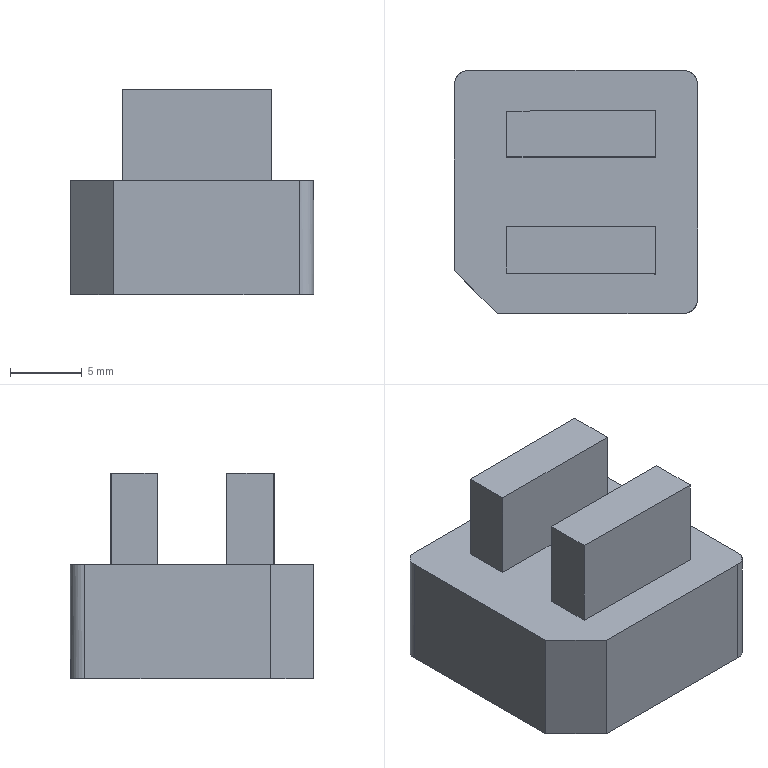NC program | PowerMill | posted with a generic post | part box 17 x 17 x 14.396 mm
Lines 1 to 1014 of 42940:
%
O0001
N104 ( POWERMILL CB  : 2026004.0)
N105 ( POST VER      : 2026.0.0.5161)
N106 ( OPTION FILE   : FANUC)
N107 ( OUTPUT WORKPLANE : WORLD)
N108 (  )
N109 ( TOOL LIST )
N110 (---------------------------------------)
N111 ( NO. | ID        | DIA.| TIP RAD|LENGTH)
N112 (---------------------------------------)
N113 (    1|D10C_1_1   |10.0 |  0.0   |69.84 )
N114 (   15|D3C_2_1    | 3.0 |  0.0   |61.44 )
N115 (    3|D10_1_1    |10.0 |  0.0   |69.56 )
N116 (   10|D3_3       | 3.0 |  0.0   |61.44 )
N117 (   13|TEXT_D4_1_1| 4.0 |  0.3   |61.64 )
N118 (---------------------------------------)
N119 (  )
N120 ( NUMBER OF TOOLPATHS: 11.0 )
N121 ( ESTIMATED PROGRAM DURATION: 0 HOURS 8 MIN 50 SEC)
N122 (  )
N123 G00 G21 G80 G40 G17
N124 G90
N125 G54
N126 G53 Z0.0
N127 (---------------)
N128 ( START TOOLPATH : 粗公开粗01-扫面平行-D10C )
N129 (---------------)
N130 ( TOOL NO.    :1 )
N131 ( TOOL TYPE   : ENDMILL)
N132 ( TOOL ID     : D10C_1_1)
N133 ( TOOL DIA    : 10.0 LENGTH 69.84)
N134 T1
N135 M6
N136 S8000 M03
N137 G00 G90 X0.0 Y0.0
N138 G43 Z10.2 H1
N139
N140 G05 P10000 R4
N141 X16.15 Y11.15
N142 Z1.198
N143 G01 Z-0.002 F6000.0
N144 X11.15 F10000.0
N145 X-11.15
N146 Y5.575
N147 X11.15
N148 Y0.0
N149 X-11.15
N150 Y-5.575
N151 X11.15
N152 Y-11.15
N153 X-11.15
N154 X-16.15
N155 Z-0.204
N156 X-11.15
N157 X11.15
N158 Y-5.575
N159 X-11.15
N160 Y0.0
N161 X11.15
N162 Y5.575
N163 X-11.15
N164 Y11.15
N165 X11.15
N166 X16.15
N167 G00 Z10.2
N168 G05 P0
N169 (---------------)
N170 ( END TOOLPATH : 粗公开粗01-扫面平行-D10C )
N171 (---------------)
N172 ( START TOOLPATH : 粗公开粗01-外形偏置-D10C )
N173 (---------------)
N174 G00 X0.3365 Y-0.0255 Z9.7958
N175 G05 P10000 R4
N176 X18.472 Y10.1346
N177 Z0.5587
N178 G01 Z-0.6413 F6000.0
N179 X17.9445 F10000.0
N180 G03 X13.197 Y5.3871 I0.0 J-4.7475
N181 G01 Y-12.389
N182 G02 X12.197 Y-13.389 I-1.0 J0.0
N183 G01 X-11.524
N184 G02 X-12.524 Y-12.389 I0.0 J1.0
N185 G01 Y12.338
N186 G02 X-11.524 Y13.338 I1.0 J0.0
N187 G01 X12.197
N188 G02 X13.197 Y12.338 I0.0 J-1.0
N189 G01 Y5.3871
N190 X10.6981 Y5.3885
N191 X10.6964 Y2.2948
N192 X10.6174 Y1.5214
N193 X10.4159 Y0.7479
N194 X10.2648 Y0.3616
N195 X10.1893 Y0.2061
N196 G03 X10.1798 Y-0.21 I0.4498 J-0.2184
N197 G01 X10.4333 Y-0.7989
N198 X10.6263 Y-1.5724
N199 X10.6974 Y-2.3458
N200 X10.6981 Y-5.4395
N201 X10.6763 Y-6.2129
N202 X10.5449 Y-6.9863
N203 X10.2853 Y-7.7598
N204 X10.0043 Y-8.321
N205 X9.8745 Y-8.5332
N206 X9.2627 Y-9.3066
N207 X8.4575 Y-9.9889
N208 X7.6841 Y-10.4256
N209 X6.9106 Y-10.7059
N210 X6.1554 Y-10.8535
N211 X5.3638 Y-10.8885
N212 X-4.6908 Y-10.8359
N213 X-5.4642 Y-10.8011
N214 X-6.2376 Y-10.6516
N215 X-7.0111 Y-10.3714
N216 X-7.5603 Y-10.08
N217 X-7.7845 Y-9.9351
N218 X-8.5375 Y-9.3066
N219 X-9.1668 Y-8.5332
N220 X-9.3313 Y-8.2684
N221 X-9.5897 Y-7.7598
N222 X-9.859 Y-6.9863
N223 X-9.9991 Y-6.2129
N224 X-10.0262 Y-5.4395
N225 X-10.0256 Y-2.3458
N226 X-9.9545 Y-1.5724
N227 X-9.7614 Y-0.7989
N228 X-9.479 Y-0.1522
N229 G03 X-9.4779 Y0.2454 I-0.4582 J0.2
N230 G01 X-9.694 Y0.7479
N231 X-9.8955 Y1.5214
N232 X-9.9744 Y2.2948
N233 X-9.9763 Y5.3885
N234 X-9.9493 Y6.1619
N235 X-9.8094 Y6.9353
N236 X-9.5404 Y7.7088
N237 X-9.3313 Y8.1307
N238 X-9.1178 Y8.4822
N239 X-8.5579 Y9.1846
N240 X-7.7845 Y9.8509
N241 X-7.5128 Y10.029
N242 X-7.0111 Y10.2989
N243 X-6.2376 Y10.5882
N244 X-5.4642 Y10.7457
N245 X-4.6908 Y10.7861
N246 X5.3638 Y10.8387
N247 X6.1372 Y10.8058
N248 X6.9106 Y10.6561
N249 X7.6841 Y10.3758
N250 X8.4575 Y9.9391
N251 X9.2309 Y9.2896
N252 X9.8753 Y8.4822
N253 X10.0043 Y8.2713
N254 X10.2859 Y7.7088
N255 X10.5452 Y6.9353
N256 X10.6764 Y6.1619
N257 X10.6981 Y5.3885
N258 X13.197 Y5.3871
N259 G00 Z3.2215
N260 G01 X18.472 Y10.1346
N261 G00 Z0.1715
N262 G01 Z-1.0285 F6000.0
N263 X17.9445 F10000.0
N264 G03 X13.197 Y5.3871 I0.0 J-4.7475
N265 G01 Y-12.389
N266 G02 X12.197 Y-13.389 I-1.0 J0.0
N267 G01 X-11.524
N268 G02 X-12.524 Y-12.389 I0.0 J1.0
N269 G01 Y12.338
N270 G02 X-11.524 Y13.338 I1.0 J0.0
N271 G01 X12.197
N272 G02 X13.197 Y12.338 I0.0 J-1.0
N273 G01 Y5.3871
N274 X10.6981 Y5.3885
N275 X10.6964 Y2.2948
N276 X10.6174 Y1.5214
N277 X10.4159 Y0.7479
N278 X10.2648 Y0.3616
N279 X10.1893 Y0.2061
N280 G03 X10.1798 Y-0.21 I0.4498 J-0.2184
N281 G01 X10.4334 Y-0.7989
N282 X10.6263 Y-1.5724
N283 X10.6974 Y-2.3458
N284 X10.6981 Y-5.4395
N285 X10.6763 Y-6.2129
N286 X10.5449 Y-6.9863
N287 X10.2853 Y-7.7598
N288 X10.0043 Y-8.321
N289 X9.8745 Y-8.5332
N290 X9.2627 Y-9.3066
N291 X8.4575 Y-9.9889
N292 X7.6841 Y-10.4256
N293 X6.9106 Y-10.7059
N294 X6.1554 Y-10.8535
N295 X5.3638 Y-10.8885
N296 X-4.6908 Y-10.8359
N297 X-5.4642 Y-10.8011
N298 X-6.2376 Y-10.6516
N299 X-7.0111 Y-10.3714
N300 X-7.5603 Y-10.08
N301 X-7.7845 Y-9.9351
N302 X-8.5375 Y-9.3066
N303 X-9.1668 Y-8.5332
N304 X-9.3313 Y-8.2684
N305 X-9.5897 Y-7.7598
N306 X-9.859 Y-6.9863
N307 X-9.9991 Y-6.2129
N308 X-10.0263 Y-5.4395
N309 X-10.0256 Y-2.3458
N310 X-9.9545 Y-1.5724
N311 X-9.7614 Y-0.7989
N312 X-9.479 Y-0.1522
N313 G03 X-9.4779 Y0.2454 I-0.4582 J0.2
N314 G01 X-9.694 Y0.7479
N315 X-9.8956 Y1.5214
N316 X-9.9744 Y2.2948
N317 X-9.9763 Y5.3885
N318 X-9.9493 Y6.1619
N319 X-9.8094 Y6.9353
N320 X-9.5404 Y7.7088
N321 X-9.3313 Y8.1307
N322 X-9.1178 Y8.4822
N323 X-8.5579 Y9.1846
N324 X-7.7845 Y9.8509
N325 X-7.5128 Y10.029
N326 X-7.0111 Y10.2989
N327 X-6.2376 Y10.5882
N328 X-5.4642 Y10.7457
N329 X-4.6908 Y10.7861
N330 X5.3638 Y10.8387
N331 X6.1372 Y10.8058
N332 X6.9106 Y10.6561
N333 X7.6841 Y10.3758
N334 X8.4575 Y9.9392
N335 X9.2309 Y9.2896
N336 X9.8753 Y8.4822
N337 X10.0043 Y8.2713
N338 X10.2859 Y7.7088
N339 X10.5452 Y6.9353
N340 X10.6764 Y6.1619
N341 X10.6981 Y5.3885
N342 X13.197 Y5.3871
N343 G00 Z2.8342
N344 G01 X18.472 Y10.1346
N345 G00 Z-0.2158
N346 G01 Z-1.4158 F6000.0
N347 X17.9445 F10000.0
N348 G03 X13.197 Y5.3871 I0.0 J-4.7475
N349 G01 Y-12.389
N350 G02 X12.197 Y-13.389 I-1.0 J0.0
N351 G01 X-11.524
N352 G02 X-12.524 Y-12.389 I0.0 J1.0
N353 G01 Y12.338
N354 G02 X-11.524 Y13.338 I1.0 J0.0
N355 G01 X12.197
N356 G02 X13.197 Y12.338 I0.0 J-1.0
N357 G01 Y5.3871
N358 X10.6981 Y5.3885
N359 X10.6964 Y2.2948
N360 X10.6174 Y1.5214
N361 X10.4159 Y0.7479
N362 X10.2648 Y0.3616
N363 X10.1893 Y0.2061
N364 G03 X10.1798 Y-0.2101 I0.4498 J-0.2184
N365 G01 X10.4334 Y-0.7989
N366 X10.6263 Y-1.5724
N367 X10.6974 Y-2.3458
N368 X10.6981 Y-5.4395
N369 X10.6763 Y-6.2129
N370 X10.5449 Y-6.9863
N371 X10.2853 Y-7.7598
N372 X10.0043 Y-8.321
N373 X9.8745 Y-8.5332
N374 X9.2627 Y-9.3066
N375 X8.4575 Y-9.9889
N376 X7.6841 Y-10.4256
N377 X6.9106 Y-10.7059
N378 X6.1554 Y-10.8535
N379 X5.3638 Y-10.8885
N380 X-4.6908 Y-10.8359
N381 X-5.4642 Y-10.8011
N382 X-6.2376 Y-10.6516
N383 X-7.0111 Y-10.3715
N384 X-7.5603 Y-10.08
N385 X-7.7845 Y-9.9351
N386 X-8.5375 Y-9.3066
N387 X-9.1668 Y-8.5332
N388 X-9.3313 Y-8.2684
N389 X-9.5897 Y-7.7598
N390 X-9.8591 Y-6.9863
N391 X-9.9991 Y-6.2129
N392 X-10.0263 Y-5.4395
N393 X-10.0256 Y-2.3458
N394 X-9.9545 Y-1.5724
N395 X-9.7614 Y-0.7989
N396 X-9.479 Y-0.1522
N397 G03 X-9.4779 Y0.2454 I-0.4582 J0.2
N398 G01 X-9.694 Y0.7479
N399 X-9.8956 Y1.5214
N400 X-9.9744 Y2.2948
N401 X-9.9763 Y5.3885
N402 X-9.9493 Y6.1619
N403 X-9.8094 Y6.9353
N404 X-9.5404 Y7.7088
N405 X-9.3313 Y8.1307
N406 X-9.1178 Y8.4822
N407 X-8.5579 Y9.1846
N408 X-7.7845 Y9.8509
N409 X-7.5128 Y10.029
N410 X-7.0111 Y10.299
N411 X-6.2376 Y10.5882
N412 X-5.4642 Y10.7457
N413 X-4.6908 Y10.7861
N414 X5.3638 Y10.8387
N415 X6.1372 Y10.8058
N416 X6.9106 Y10.6561
N417 X7.6841 Y10.3758
N418 X8.4575 Y9.9392
N419 X9.2309 Y9.2896
N420 X9.8753 Y8.4822
N421 X10.0043 Y8.2713
N422 X10.2859 Y7.7088
N423 X10.5452 Y6.9353
N424 X10.6764 Y6.1619
N425 X10.6981 Y5.3885
N426 X13.197 Y5.3871
N427 G00 Z2.447
N428 G01 X18.472 Y10.1346
N429 G00 Z-0.603
N430 G01 Z-1.803 F6000.0
N431 X17.9445 F10000.0
N432 G03 X13.197 Y5.3871 I0.0 J-4.7475
N433 G01 Y-12.389
N434 G02 X12.197 Y-13.389 I-1.0 J0.0
N435 G01 X-11.524
N436 G02 X-12.524 Y-12.389 I0.0 J1.0
N437 G01 Y12.338
N438 G02 X-11.524 Y13.338 I1.0 J0.0
N439 G01 X12.197
N440 G02 X13.197 Y12.338 I0.0 J-1.0
N441 G01 Y5.3871
N442 X10.6981 Y5.3885
N443 X10.6964 Y2.2948
N444 X10.6174 Y1.5214
N445 X10.4159 Y0.7479
N446 X10.2648 Y0.3616
N447 X10.1893 Y0.2061
N448 G03 X10.1798 Y-0.2101 I0.4498 J-0.2184
N449 G01 X10.4334 Y-0.7989
N450 X10.6263 Y-1.5724
N451 X10.6974 Y-2.3458
N452 X10.6981 Y-5.4395
N453 X10.6763 Y-6.2129
N454 X10.545 Y-6.9863
N455 X10.2853 Y-7.7598
N456 X10.0043 Y-8.321
N457 X9.8745 Y-8.5332
N458 X9.2627 Y-9.3066
N459 X8.4575 Y-9.9889
N460 X7.6841 Y-10.4256
N461 X6.9106 Y-10.7059
N462 X6.1554 Y-10.8535
N463 X5.3638 Y-10.8885
N464 X-4.6908 Y-10.8359
N465 X-5.4642 Y-10.8011
N466 X-6.2376 Y-10.6516
N467 X-7.0111 Y-10.3715
N468 X-7.5603 Y-10.08
N469 X-7.7845 Y-9.9351
N470 X-8.5375 Y-9.3066
N471 X-9.1668 Y-8.5332
N472 X-9.3313 Y-8.2684
N473 X-9.5897 Y-7.7598
N474 X-9.8591 Y-6.9863
N475 X-9.9991 Y-6.2129
N476 X-10.0263 Y-5.4395
N477 X-10.0256 Y-2.3458
N478 X-9.9545 Y-1.5724
N479 X-9.7614 Y-0.7989
N480 X-9.479 Y-0.1522
N481 G03 X-9.4779 Y0.2454 I-0.4582 J0.2
N482 G01 X-9.694 Y0.7479
N483 X-9.8956 Y1.5214
N484 X-9.9745 Y2.2948
N485 X-9.9763 Y5.3885
N486 X-9.9493 Y6.1619
N487 X-9.8094 Y6.9353
N488 X-9.5404 Y7.7088
N489 X-9.3313 Y8.1307
N490 X-9.1178 Y8.4822
N491 X-8.5579 Y9.1846
N492 X-7.7845 Y9.8509
N493 X-7.5128 Y10.029
N494 X-7.0111 Y10.299
N495 X-6.2376 Y10.5882
N496 X-5.4642 Y10.7457
N497 X-4.6908 Y10.7861
N498 X5.3638 Y10.8387
N499 X6.1372 Y10.8058
N500 X6.9106 Y10.6561
N501 X7.6841 Y10.3758
N502 X8.4575 Y9.9392
N503 X9.2309 Y9.2896
N504 X9.8753 Y8.4822
N505 X10.0043 Y8.2713
N506 X10.2859 Y7.7088
N507 X10.5452 Y6.9353
N508 X10.6764 Y6.1619
N509 X10.6981 Y5.3885
N510 X13.197 Y5.3871
N511 G00 Z2.0598
N512 G01 X18.472 Y10.1346
N513 G00 Z-0.9902
N514 G01 Z-2.1902 F6000.0
N515 X17.9445 F10000.0
N516 G03 X13.197 Y5.3871 I0.0 J-4.7475
N517 G01 Y-12.389
N518 G02 X12.197 Y-13.389 I-1.0 J0.0
N519 G01 X-11.524
N520 G02 X-12.524 Y-12.389 I0.0 J1.0
N521 G01 Y12.338
N522 G02 X-11.524 Y13.338 I1.0 J0.0
N523 G01 X12.197
N524 G02 X13.197 Y12.338 I0.0 J-1.0
N525 G01 Y5.3871
N526 X10.6981 Y5.3885
N527 X10.6964 Y2.2948
N528 X10.6174 Y1.5214
N529 X10.4159 Y0.7479
N530 X10.2648 Y0.3616
N531 X10.1893 Y0.2061
N532 G03 X10.1798 Y-0.2101 I0.4498 J-0.2184
N533 G01 X10.4334 Y-0.7989
N534 X10.6264 Y-1.5724
N535 X10.6975 Y-2.3458
N536 X10.6981 Y-5.4395
N537 X10.6763 Y-6.2129
N538 X10.545 Y-6.9863
N539 X10.2853 Y-7.7598
N540 X10.0043 Y-8.321
N541 X9.8745 Y-8.5332
N542 X9.2627 Y-9.3066
N543 X8.4575 Y-9.9889
N544 X7.6841 Y-10.4256
N545 X6.9106 Y-10.7059
N546 X6.1554 Y-10.8535
N547 X5.3638 Y-10.8885
N548 X-4.6908 Y-10.8359
N549 X-5.4642 Y-10.8011
N550 X-6.2376 Y-10.6516
N551 X-7.0111 Y-10.3715
N552 X-7.5603 Y-10.08
N553 X-7.7845 Y-9.9351
N554 X-8.5375 Y-9.3066
N555 X-9.1668 Y-8.5332
N556 X-9.3313 Y-8.2684
N557 X-9.5897 Y-7.7598
N558 X-9.8591 Y-6.9863
N559 X-9.9991 Y-6.2129
N560 X-10.0263 Y-5.4395
N561 X-10.0256 Y-2.3458
N562 X-9.9545 Y-1.5724
N563 X-9.7614 Y-0.7989
N564 X-9.479 Y-0.1522
N565 G03 X-9.4779 Y0.2454 I-0.4582 J0.2
N566 G01 X-9.694 Y0.7479
N567 X-9.8956 Y1.5214
N568 X-9.9745 Y2.2948
N569 X-9.9763 Y5.3885
N570 X-9.9493 Y6.1619
N571 X-9.8094 Y6.9353
N572 X-9.5404 Y7.7088
N573 X-9.3313 Y8.1307
N574 X-9.1179 Y8.4822
N575 X-8.5579 Y9.1846
N576 X-7.7845 Y9.8509
N577 X-7.5129 Y10.029
N578 X-7.0111 Y10.299
N579 X-6.2376 Y10.5882
N580 X-5.4642 Y10.7457
N581 X-4.6908 Y10.7861
N582 X5.3638 Y10.8387
N583 X6.1372 Y10.8058
N584 X6.9106 Y10.6561
N585 X7.6841 Y10.3758
N586 X8.4575 Y9.9392
N587 X9.2309 Y9.2896
N588 X9.8753 Y8.4822
N589 X10.0043 Y8.2713
N590 X10.2859 Y7.7088
N591 X10.5452 Y6.9353
N592 X10.6764 Y6.1619
N593 X10.6981 Y5.3885
N594 X13.197 Y5.3871
N595 G00 Z1.6725
N596 G01 X18.472 Y10.1346
N597 G00 Z-1.3775
N598 G01 Z-2.5775 F6000.0
N599 X17.9445 F10000.0
N600 G03 X13.197 Y5.3871 I0.0 J-4.7475
N601 G01 Y-12.389
N602 G02 X12.197 Y-13.389 I-1.0 J0.0
N603 G01 X-11.524
N604 G02 X-12.524 Y-12.389 I0.0 J1.0
N605 G01 Y12.338
N606 G02 X-11.524 Y13.338 I1.0 J0.0
N607 G01 X12.197
N608 G02 X13.197 Y12.338 I0.0 J-1.0
N609 G01 Y5.3871
N610 X10.6982 Y5.3885
N611 X10.6964 Y2.2948
N612 X10.6174 Y1.5214
N613 X10.4159 Y0.7479
N614 X10.2648 Y0.3616
N615 X10.1893 Y0.2061
N616 G03 X10.1798 Y-0.2101 I0.4498 J-0.2184
N617 G01 X10.4334 Y-0.7989
N618 X10.6264 Y-1.5724
N619 X10.6975 Y-2.3458
N620 X10.6982 Y-5.4395
N621 X10.6764 Y-6.2129
N622 X10.545 Y-6.9863
N623 X10.2853 Y-7.7598
N624 X10.0043 Y-8.321
N625 X9.8745 Y-8.5332
N626 X9.2627 Y-9.3066
N627 X8.4575 Y-9.989
N628 X7.6841 Y-10.4256
N629 X6.9106 Y-10.7059
N630 X6.1554 Y-10.8535
N631 X5.3638 Y-10.8885
N632 X-4.6908 Y-10.8359
N633 X-5.4642 Y-10.8012
N634 X-6.2376 Y-10.6516
N635 X-7.0111 Y-10.3715
N636 X-7.5603 Y-10.08
N637 X-7.7845 Y-9.9351
N638 X-8.5375 Y-9.3066
N639 X-9.1668 Y-8.5332
N640 X-9.3313 Y-8.2684
N641 X-9.5897 Y-7.7598
N642 X-9.8591 Y-6.9863
N643 X-9.9991 Y-6.2129
N644 X-10.0263 Y-5.4395
N645 X-10.0256 Y-2.3458
N646 X-9.9545 Y-1.5724
N647 X-9.7614 Y-0.7989
N648 X-9.479 Y-0.1523
N649 G03 X-9.4779 Y0.2454 I-0.4582 J0.2001
N650 G01 X-9.694 Y0.7479
N651 X-9.8956 Y1.5214
N652 X-9.9745 Y2.2948
N653 X-9.9763 Y5.3885
N654 X-9.9493 Y6.1619
N655 X-9.8094 Y6.9353
N656 X-9.5404 Y7.7088
N657 X-9.3313 Y8.1307
N658 X-9.1179 Y8.4822
N659 X-8.5579 Y9.1846
N660 X-7.7845 Y9.8509
N661 X-7.5129 Y10.029
N662 X-7.0111 Y10.299
N663 X-6.2376 Y10.5882
N664 X-5.4642 Y10.7457
N665 X-4.6908 Y10.7861
N666 X5.3638 Y10.8388
N667 X6.1372 Y10.8059
N668 X6.9106 Y10.6562
N669 X7.6841 Y10.3758
N670 X8.4575 Y9.9392
N671 X9.2309 Y9.2896
N672 X9.8753 Y8.4822
N673 X10.0043 Y8.2713
N674 X10.2859 Y7.7088
N675 X10.5452 Y6.9353
N676 X10.6764 Y6.1619
N677 X10.6982 Y5.3885
N678 X13.197 Y5.3871
N679 G00 Z1.2852
N680 G01 X18.472 Y10.1346
N681 G00 Z-1.7648
N682 G01 Z-2.9648 F6000.0
N683 X17.9445 F10000.0
N684 G03 X13.197 Y5.3871 I0.0 J-4.7475
N685 G01 Y-12.389
N686 G02 X12.197 Y-13.389 I-1.0 J0.0
N687 G01 X-11.524
N688 G02 X-12.524 Y-12.389 I0.0 J1.0
N689 G01 Y12.338
N690 G02 X-11.524 Y13.338 I1.0 J0.0
N691 G01 X12.197
N692 G02 X13.197 Y12.338 I0.0 J-1.0
N693 G01 Y5.3871
N694 X10.6982 Y5.3885
N695 X10.6964 Y2.2948
N696 X10.6175 Y1.5214
N697 X10.4159 Y0.7479
N698 X10.2648 Y0.3616
N699 X10.1893 Y0.2061
N700 G03 X10.1798 Y-0.2101 I0.4498 J-0.2184
N701 G01 X10.4334 Y-0.7989
N702 X10.6264 Y-1.5724
N703 X10.6975 Y-2.3458
N704 X10.6982 Y-5.4395
N705 X10.6764 Y-6.2129
N706 X10.545 Y-6.9863
N707 X10.2853 Y-7.7598
N708 X10.0043 Y-8.321
N709 X9.8745 Y-8.5332
N710 X9.2627 Y-9.3066
N711 X8.4575 Y-9.989
N712 X7.6841 Y-10.4256
N713 X6.9106 Y-10.7059
N714 X6.1555 Y-10.8535
N715 X5.3638 Y-10.8885
N716 X-4.6908 Y-10.8359
N717 X-5.4642 Y-10.8012
N718 X-6.2376 Y-10.6516
N719 X-7.0111 Y-10.3715
N720 X-7.5603 Y-10.08
N721 X-7.7845 Y-9.9351
N722 X-8.5375 Y-9.3066
N723 X-9.1668 Y-8.5332
N724 X-9.3313 Y-8.2684
N725 X-9.5897 Y-7.7598
N726 X-9.8591 Y-6.9863
N727 X-9.9991 Y-6.2129
N728 X-10.0263 Y-5.4395
N729 X-10.0256 Y-2.3458
N730 X-9.9545 Y-1.5724
N731 X-9.7614 Y-0.7989
N732 X-9.479 Y-0.1523
N733 G03 X-9.4779 Y0.2454 I-0.4582 J0.2001
N734 G01 X-9.694 Y0.7479
N735 X-9.8956 Y1.5214
N736 X-9.9745 Y2.2948
N737 X-9.9763 Y5.3885
N738 X-9.9493 Y6.1619
N739 X-9.8094 Y6.9353
N740 X-9.5404 Y7.7088
N741 X-9.3313 Y8.1307
N742 X-9.1179 Y8.4822
N743 X-8.5579 Y9.1846
N744 X-7.7845 Y9.8509
N745 X-7.5129 Y10.029
N746 X-7.0111 Y10.299
N747 X-6.2376 Y10.5882
N748 X-5.4642 Y10.7457
N749 X-4.6908 Y10.7861
N750 X5.3638 Y10.8388
N751 X6.1372 Y10.8059
N752 X6.9106 Y10.6562
N753 X7.6841 Y10.3758
N754 X8.4575 Y9.9392
N755 X9.2309 Y9.2896
N756 X9.8753 Y8.4822
N757 X10.0043 Y8.2714
N758 X10.2859 Y7.7088
N759 X10.5452 Y6.9353
N760 X10.6764 Y6.1619
N761 X10.6982 Y5.3885
N762 X13.197 Y5.3871
N763 G00 Z0.898
N764 G01 X18.472 Y10.1346
N765 G00 Z-2.152
N766 G01 Z-3.352 F6000.0
N767 X17.9445 F10000.0
N768 G03 X13.197 Y5.3871 I0.0 J-4.7475
N769 G01 Y-12.389
N770 G02 X12.197 Y-13.389 I-1.0 J0.0
N771 G01 X-11.524
N772 G02 X-12.524 Y-12.389 I0.0 J1.0
N773 G01 Y12.338
N774 G02 X-11.524 Y13.338 I1.0 J0.0
N775 G01 X12.197
N776 G02 X13.197 Y12.338 I0.0 J-1.0
N777 G01 Y5.3871
N778 X10.6982 Y5.3885
N779 X10.6964 Y2.2948
N780 X10.6175 Y1.5214
N781 X10.4159 Y0.7479
N782 X10.2648 Y0.3616
N783 X10.1893 Y0.2061
N784 G03 X10.1798 Y-0.2101 I0.4498 J-0.2184
N785 G01 X10.4334 Y-0.7989
N786 X10.6264 Y-1.5724
N787 X10.6975 Y-2.3458
N788 X10.6982 Y-5.4395
N789 X10.6764 Y-6.2129
N790 X10.545 Y-6.9863
N791 X10.2853 Y-7.7598
N792 X10.0043 Y-8.3211
N793 X9.8745 Y-8.5332
N794 X9.2627 Y-9.3066
N795 X8.4575 Y-9.989
N796 X7.6841 Y-10.4256
N797 X6.9106 Y-10.7059
N798 X6.1555 Y-10.8535
N799 X5.3638 Y-10.8885
N800 X-4.6908 Y-10.8359
N801 X-5.4642 Y-10.8012
N802 X-6.2376 Y-10.6516
N803 X-7.0111 Y-10.3715
N804 X-7.5604 Y-10.08
N805 X-7.7845 Y-9.9351
N806 X-8.5375 Y-9.3066
N807 X-9.1668 Y-8.5332
N808 X-9.3313 Y-8.2684
N809 X-9.5897 Y-7.7598
N810 X-9.8591 Y-6.9863
N811 X-9.9991 Y-6.2129
N812 X-10.0263 Y-5.4395
N813 X-10.0256 Y-2.3458
N814 X-9.9545 Y-1.5724
N815 X-9.7614 Y-0.7989
N816 X-9.479 Y-0.1523
N817 G03 X-9.4779 Y0.2454 I-0.4583 J0.2001
N818 G01 X-9.694 Y0.7479
N819 X-9.8956 Y1.5214
N820 X-9.9745 Y2.2948
N821 X-9.9763 Y5.3885
N822 X-9.9493 Y6.1619
N823 X-9.8094 Y6.9353
N824 X-9.5404 Y7.7088
N825 X-9.3313 Y8.1307
N826 X-9.1179 Y8.4822
N827 X-8.5579 Y9.1846
N828 X-7.7845 Y9.8509
N829 X-7.5129 Y10.029
N830 X-7.0111 Y10.299
N831 X-6.2376 Y10.5882
N832 X-5.4642 Y10.7457
N833 X-4.6908 Y10.7861
N834 X5.3638 Y10.8388
N835 X6.1372 Y10.8059
N836 X6.9106 Y10.6562
N837 X7.6841 Y10.3758
N838 X8.4575 Y9.9392
N839 X9.2309 Y9.2897
N840 X9.8753 Y8.4822
N841 X10.0043 Y8.2714
N842 X10.2859 Y7.7088
N843 X10.5452 Y6.9353
N844 X10.6765 Y6.1619
N845 X10.6982 Y5.3885
N846 X13.197 Y5.3871
N847 G00 Z0.5108
N848 G01 X18.472 Y10.1346
N849 G00 Z-2.5392
N850 G01 Z-3.7392 F6000.0
N851 X17.9445 F10000.0
N852 G03 X13.197 Y5.3871 I0.0 J-4.7475
N853 G01 Y-12.389
N854 G02 X12.197 Y-13.389 I-1.0 J0.0
N855 G01 X-11.524
N856 G02 X-12.524 Y-12.389 I0.0 J1.0
N857 G01 Y12.338
N858 G02 X-11.524 Y13.338 I1.0 J0.0
N859 G01 X12.197
N860 G02 X13.197 Y12.338 I0.0 J-1.0
N861 G01 Y5.3871
N862 X10.6982 Y5.3885
N863 X10.6964 Y2.2948
N864 X10.6175 Y1.5214
N865 X10.4159 Y0.7479
N866 X10.2648 Y0.3616
N867 X10.1893 Y0.2061
N868 G03 X10.1798 Y-0.2101 I0.4498 J-0.2184
N869 G01 X10.4334 Y-0.7989
N870 X10.6264 Y-1.5724
N871 X10.6975 Y-2.3458
N872 X10.6982 Y-5.4395
N873 X10.6764 Y-6.2129
N874 X10.545 Y-6.9863
N875 X10.2853 Y-7.7598
N876 X10.0043 Y-8.3211
N877 X9.8745 Y-8.5332
N878 X9.2627 Y-9.3066
N879 X8.4575 Y-9.989
N880 X7.6841 Y-10.4256
N881 X6.9106 Y-10.706
N882 X6.1555 Y-10.8535
N883 X5.3638 Y-10.8885
N884 X-4.6908 Y-10.8359
N885 X-5.4642 Y-10.8012
N886 X-6.2376 Y-10.6516
N887 X-7.0111 Y-10.3715
N888 X-7.5604 Y-10.08
N889 X-7.7845 Y-9.9351
N890 X-8.5375 Y-9.3066
N891 X-9.1668 Y-8.5332
N892 X-9.3313 Y-8.2684
N893 X-9.5897 Y-7.7598
N894 X-9.8591 Y-6.9863
N895 X-9.9991 Y-6.2129
N896 X-10.0263 Y-5.4395
N897 X-10.0256 Y-2.3458
N898 X-9.9545 Y-1.5724
N899 X-9.7614 Y-0.7989
N900 X-9.479 Y-0.1523
N901 G03 X-9.4779 Y0.2454 I-0.4583 J0.2001
N902 G01 X-9.694 Y0.7479
N903 X-9.8956 Y1.5214
N904 X-9.9745 Y2.2948
N905 X-9.9763 Y5.3885
N906 X-9.9493 Y6.1619
N907 X-9.8094 Y6.9353
N908 X-9.5404 Y7.7088
N909 X-9.3313 Y8.1307
N910 X-9.1179 Y8.4822
N911 X-8.5579 Y9.1846
N912 X-7.7845 Y9.8509
N913 X-7.5129 Y10.029
N914 X-7.0111 Y10.299
N915 X-6.2376 Y10.5882
N916 X-5.4642 Y10.7457
N917 X-4.6908 Y10.7861
N918 X5.3638 Y10.8388
N919 X6.1372 Y10.8059
N920 X6.9106 Y10.6562
N921 X7.6841 Y10.3758
N922 X8.4575 Y9.9392
N923 X9.2309 Y9.2897
N924 X9.8753 Y8.4822
N925 X10.0043 Y8.2714
N926 X10.2859 Y7.7088
N927 X10.5452 Y6.9353
N928 X10.6765 Y6.1619
N929 X10.6982 Y5.3885
N930 X13.197 Y5.3871
N931 G00 Z0.1235
N932 G01 X18.472 Y10.1346
N933 G00 Z-2.9265
N934 G01 Z-4.1265 F6000.0
N935 X17.9445 F10000.0
N936 G03 X13.197 Y5.3871 I0.0 J-4.7475
N937 G01 Y-12.389
N938 G02 X12.197 Y-13.389 I-1.0 J0.0
N939 G01 X-11.524
N940 G02 X-12.524 Y-12.389 I0.0 J1.0
N941 G01 Y12.338
N942 G02 X-11.524 Y13.338 I1.0 J0.0
N943 G01 X12.197
N944 G02 X13.197 Y12.338 I0.0 J-1.0
N945 G01 Y5.3871
N946 X10.6982 Y5.3885
N947 X10.6964 Y2.2948
N948 X10.6175 Y1.5214
N949 X10.4159 Y0.7479
N950 X10.2648 Y0.3616
N951 X10.1893 Y0.2061
N952 G03 X10.1798 Y-0.2101 I0.4498 J-0.2184
N953 G01 X10.4334 Y-0.7989
N954 X10.6264 Y-1.5724
N955 X10.6975 Y-2.3458
N956 X10.6982 Y-5.4395
N957 X10.6764 Y-6.2129
N958 X10.545 Y-6.9863
N959 X10.2853 Y-7.7598
N960 X10.0043 Y-8.3211
N961 X9.8745 Y-8.5332
N962 X9.2627 Y-9.3066
N963 X8.4575 Y-9.989
N964 X7.6841 Y-10.4256
N965 X6.9106 Y-10.706
N966 X6.1555 Y-10.8535
N967 X5.3638 Y-10.8886
N968 X-4.6908 Y-10.8359
N969 X-5.4642 Y-10.8012
N970 X-6.2376 Y-10.6516
N971 X-7.0111 Y-10.3715
N972 X-7.5604 Y-10.08
N973 X-7.7845 Y-9.9351
N974 X-8.5376 Y-9.3066
N975 X-9.1668 Y-8.5332
N976 X-9.3313 Y-8.2684
N977 X-9.5897 Y-7.7598
N978 X-9.8591 Y-6.9863
N979 X-9.9991 Y-6.2129
N980 X-10.0263 Y-5.4395
N981 X-10.0256 Y-2.3458
N982 X-9.9545 Y-1.5724
N983 X-9.7614 Y-0.7989
N984 X-9.479 Y-0.1523
N985 G03 X-9.4779 Y0.2454 I-0.4583 J0.2001
N986 G01 X-9.6941 Y0.7479
N987 X-9.8956 Y1.5214
N988 X-9.9745 Y2.2948
N989 X-9.9763 Y5.3885
N990 X-9.9493 Y6.1619
N991 X-9.8094 Y6.9353
N992 X-9.5404 Y7.7088
N993 X-9.3313 Y8.1307
N994 X-9.1179 Y8.4822
N995 X-8.5579 Y9.1846
N996 X-7.7845 Y9.8509
N997 X-7.5129 Y10.029
N998 X-7.0111 Y10.299
N999 X-6.2376 Y10.5882
N1000 X-5.4642 Y10.7457
N1001 X-4.6908 Y10.7861
N1002 X5.3638 Y10.8388
N1003 X6.1372 Y10.8059
N1004 X6.9106 Y10.6562
N1005 X7.6841 Y10.3758
N1006 X8.4575 Y9.9392
N1007 X9.2309 Y9.2897
N1008 X9.8753 Y8.4822
N1009 X10.0043 Y8.2714
N1010 X10.2859 Y7.7088
N1011 X10.5452 Y6.9353
N1012 X10.6765 Y6.1619
N1013 X10.6982 Y5.3885
N1014 X13.197 Y5.3871
N1015 G00 Z-0.2638
N1016 G01 X18.472 Y10.1346
N1017 G00 Z-3.3138
N1018 G01 Z-4.5138 F6000.0
N1019 X17.9445 F10000.0
N1020 G03 X13.197 Y5.3871 I0.0 J-4.7475
N1021 G01 Y-12.389
N1022 G02 X12.197 Y-13.389 I-1.0 J0.0
N1023 G01 X-11.524
N1024 G02 X-12.524 Y-12.389 I0.0 J1.0
N1025 G01 Y12.338
N1026 G02 X-11.524 Y13.338 I1.0 J0.0
N1027 G01 X12.197
N1028 G02 X13.197 Y12.338 I0.0 J-1.0
N1029 G01 Y5.3871
N1030 X10.6982 Y5.3885
N1031 X10.6964 Y2.2948
N1032 X10.6175 Y1.5214
N1033 X10.4159 Y0.7479
N1034 X10.2648 Y0.3616
N1035 X10.1893 Y0.2061
N1036 G03 X10.1798 Y-0.2101 I0.4498 J-0.2184
N1037 G01 X10.4334 Y-0.7989
N1038 X10.6264 Y-1.5724
N1039 X10.6975 Y-2.3458
N1040 X10.6982 Y-5.4395
N1041 X10.6764 Y-6.2129
N1042 X10.545 Y-6.9863
N1043 X10.2853 Y-7.7598
N1044 X10.0043 Y-8.3211
N1045 X9.8745 Y-8.5332
N1046 X9.2627 Y-9.3066
N1047 X8.4575 Y-9.989
N1048 X7.6841 Y-10.4256
N1049 X6.9106 Y-10.706
N1050 X6.1555 Y-10.8535
N1051 X5.3638 Y-10.8886
N1052 X-4.6908 Y-10.8359
N1053 X-5.4642 Y-10.8012
N1054 X-6.2376 Y-10.6517
N1055 X-7.0111 Y-10.3715
N1056 X-7.5604 Y-10.08
N1057 X-7.7845 Y-9.9351
N1058 X-8.5376 Y-9.3066
N1059 X-9.1668 Y-8.5332
N1060 X-9.3313 Y-8.2684
N1061 X-9.5897 Y-7.7598
N1062 X-9.8591 Y-6.9863
N1063 X-9.9991 Y-6.2129
N1064 X-10.0263 Y-5.4395
N1065 X-10.0256 Y-2.3458
N1066 X-9.9545 Y-1.5724
N1067 X-9.7614 Y-0.7989
N1068 X-9.479 Y-0.1523
N1069 G03 X-9.4779 Y0.2454 I-0.4583 J0.2001
N1070 G01 X-9.6941 Y0.7479
N1071 X-9.8956 Y1.5214
N1072 X-9.9745 Y2.2948
N1073 X-9.9763 Y5.3885
N1074 X-9.9493 Y6.1619
N1075 X-9.8094 Y6.9353
N1076 X-9.5404 Y7.7088
N1077 X-9.3313 Y8.1307
N1078 X-9.1179 Y8.4822
N1079 X-8.5579 Y9.1846
N1080 X-7.7845 Y9.8509
N1081 X-7.5129 Y10.029
N1082 X-7.0111 Y10.299
N1083 X-6.2376 Y10.5882
N1084 X-5.4642 Y10.7457
N1085 X-4.6908 Y10.7861
N1086 X5.3638 Y10.8388
N1087 X6.1372 Y10.8059
N1088 X6.9106 Y10.6562
N1089 X7.6841 Y10.3758
N1090 X8.4575 Y9.9392
N1091 X9.2309 Y9.2897
N1092 X9.8753 Y8.4822
N1093 X10.0043 Y8.2714
N1094 X10.2859 Y7.7088
N1095 X10.5452 Y6.9353
N1096 X10.6765 Y6.1619
N1097 X10.6982 Y5.3885
N1098 X13.197 Y5.3871
N1099 G00 Z-0.651
N1100 G01 X18.472 Y10.1346
N1101 G00 Z-3.701
N1102 G01 Z-4.901 F6000.0
N1103 X17.9445 F10000.0
N1104 G03 X13.197 Y5.3871 I0.0 J-4.7475
N1105 G01 Y-12.389
N1106 G02 X12.197 Y-13.389 I-1.0 J0.0
N1107 G01 X-11.524
N1108 G02 X-12.524 Y-12.389 I0.0 J1.0
N1109 G01 Y12.338
N1110 G02 X-11.524 Y13.338 I1.0 J0.0
N1111 G01 X12.197